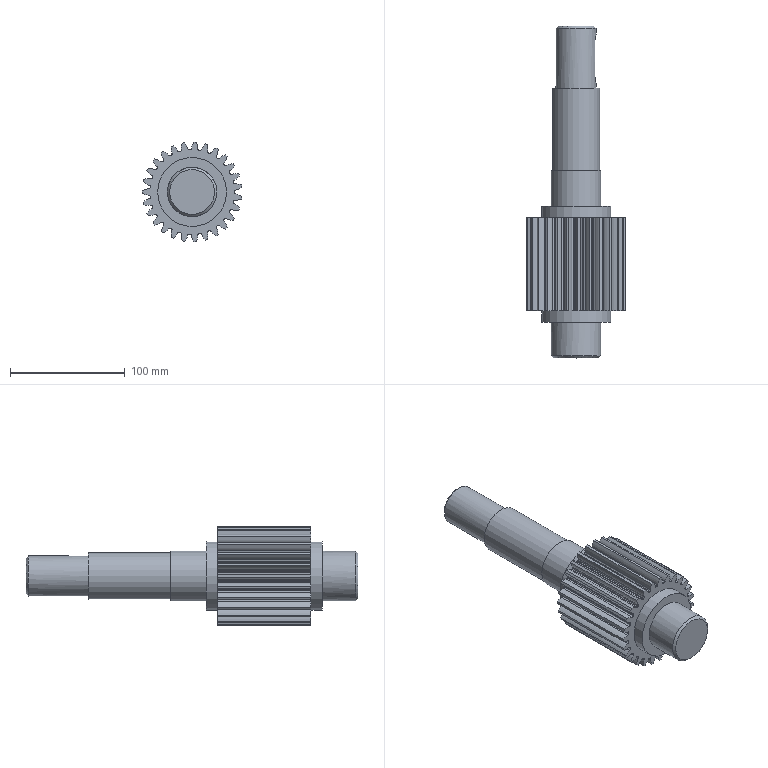Part | NX | features BREP 27, META 27, DATUM_CSYS 8, EXTRUDE 7, SKETCH 7, EXTRACT_DATUM_AXIS 4, EXTRACT_DATUM_PLANE 2, EXTRACT_STRING 2, BLEND 1, CHAMFER 1, CYLINDER 1, FSET 1, Instance Feature 1, Mirror Feature 1 | 1 solid | 183 faces | box 86.819 x 289 x 86.952 mm | volume 701275 mm3 | spline 135 | cylinder 35 | plane 11 | cone 2 | commonest cylinder face diameters 73.5 x27 12 x2 43 x2 60 x2 35 x1 41 x1